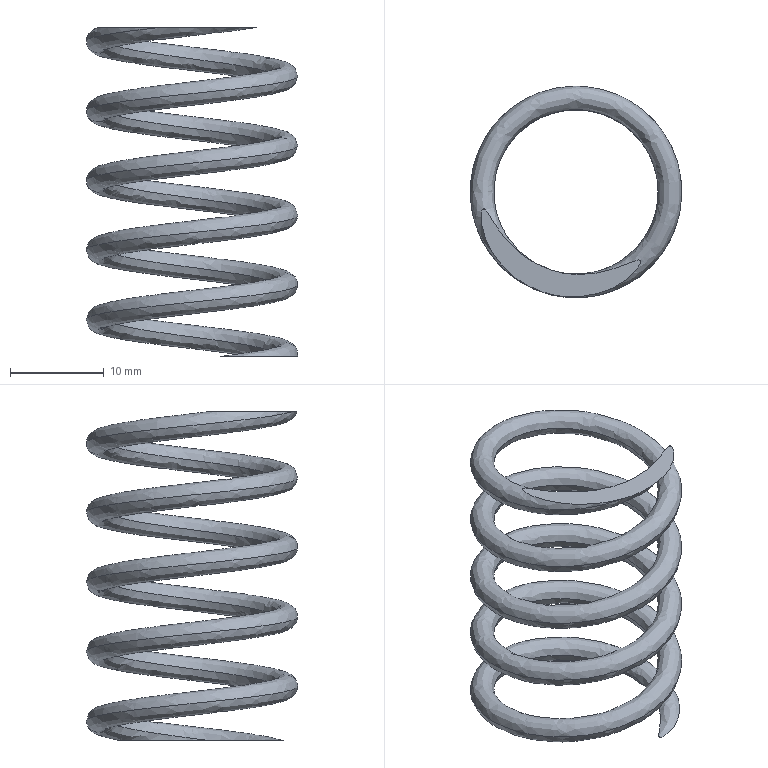Part | SolidWorks | features MirrorStock 1 | 1 solid | 4 faces | box 22.5 x 22.5 x 35 mm | volume 1475 mm3 | spline 2 | plane 2